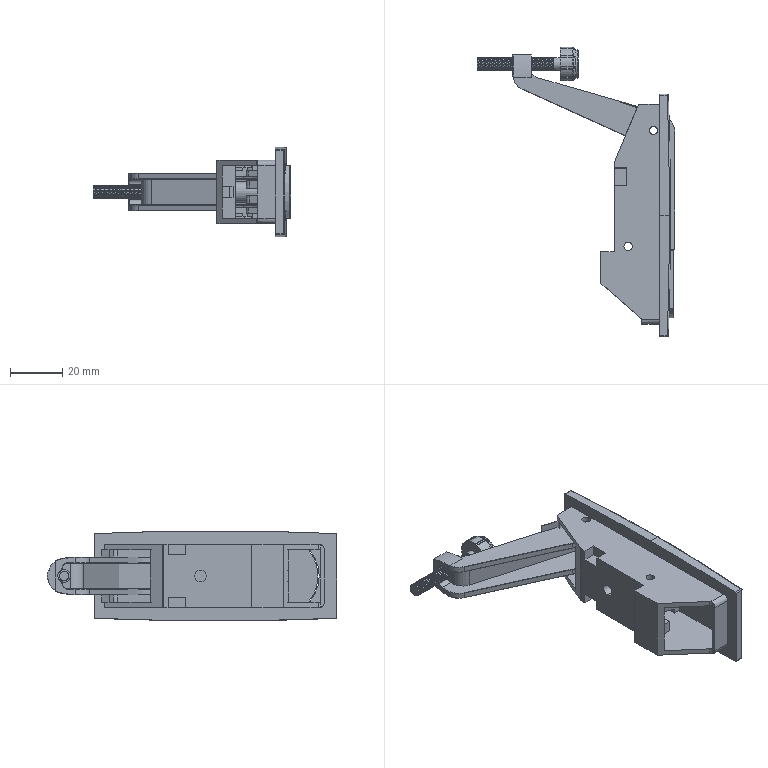Part | SolidWorks | 3 solids | 491 faces | box 75.7 x 110.704 x 34.425 mm | volume 27643 mm3 | cylinder 245 | plane 124 | spline 85 | torus 31 | sphere 4 | cone 2 | commonest cylinder face diameters 4.8 x120 0.4 x30 3.2 x14 0.692 x12 4 x10 12.8 x10